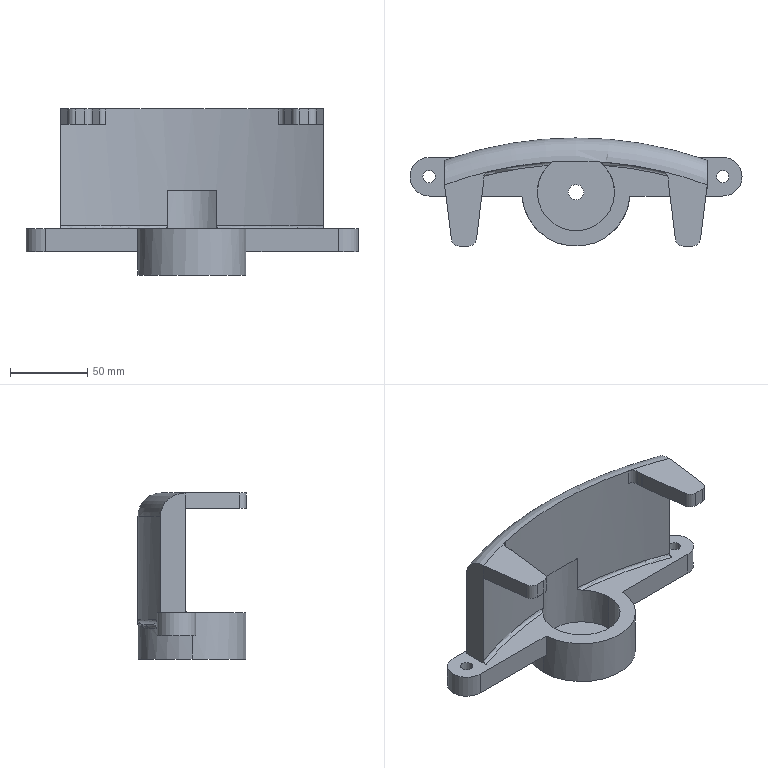Part | SolidWorks | features Fillet 5, ICE 5, Extrusion 1 | 1 solid | 68 faces | box 215 x 70 x 107.5 mm | volume 333533 mm3 | cylinder 27 | plane 26 | spline 8 | torus 7 | commonest cylinder face diameters 10 x10 6 x4 8 x4 25 x3 50 x2 70 x2